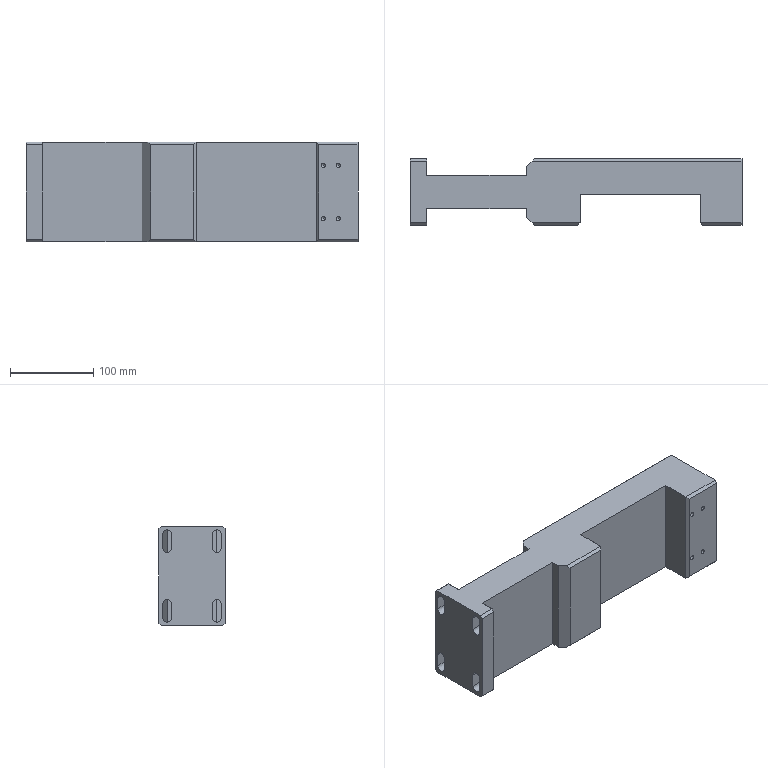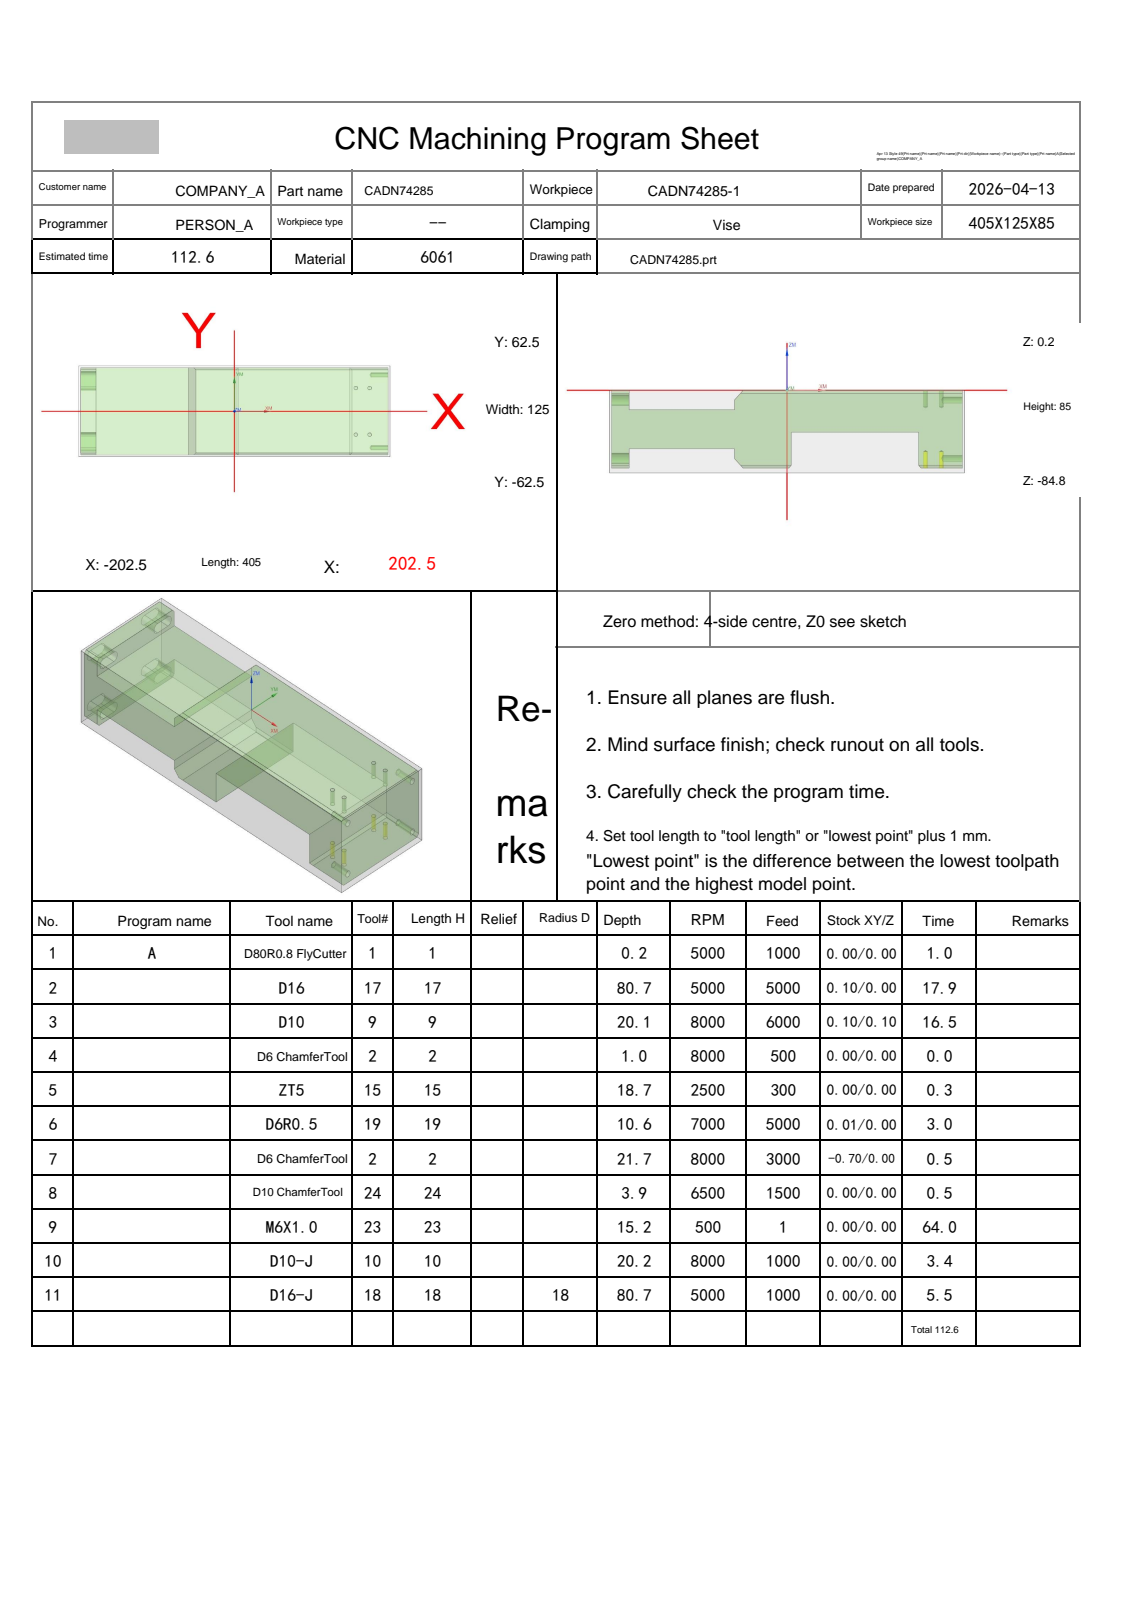NC program | NX | posted by the shop | part box 400 x 80 x 120 mm
Lines 1 to 710 of 8047:
%
O0001
(Machine time: 174.87 MIN)
(===Total Tool:10===)
(T1=D80R0.8 FlyCutter D=80.  R=0.8  D-  H01 Z=-0.   )
(T17=D16    D=16.  R=0.   D-  H17 Z=-80.5 )
(T9=D10     D=10.  R=0.   D-  H09 Z=-19.9 )
(T2=D6 ChamferTool   D=6.   R=0.   D-  H02 Z=-21.5 )
(T15=ZT5    D=5.   DR_a=118 D-  H15 Z=-18.5 )
(T19=D6R0.5 D=6.   R=0.5  D-  H19 Z=-10.4 )
(T24=D10 ChamferTool D=10.  R=0.   D-  H24 Z=-3.7  )
(T23=M6X1.0 D=5.   DR_a=180 D-  H23 Z=-15.  )
(T10=D10-J  D=10.  R=0.   D10 H10 Z=-20.  )
(T18=D16-J  D=16.  R=0.   D18 H18 Z=-80.5 )
G80 G90 G17 G49 G40
G91 G28 Z0
M01
N1 T01 M06
(D80R0.8 FlyCutter  D=80. R=0.8 H=01 ce=0.00 di=0.00)
G00 G90 G54 X245. Y-33.333 M03 S5000
G43 H01 Z20.
M08
Z2.
G01 Z0.0 F1000.
X240.
X-240.
Y33.333
X240.
X245.
Z2.
G00 Z20.
G91 G28 Z0.0
M05
M09
G91 G28 Z0.0
M01
N2 T17 M06
(D16  D=16. R=0. H=17 ce=0.10 di=0.00)
G00 G90 G54 X0.0 Y68.1 M03 S5000
G43 H17 Z20.
M08
Z.5
G01 X200. Z.317 F5000.
G02 X208.1 Y60. Z.305 I0.0 J-8.1
G01 Y-60. Z.195
G02 X200. Y-68.1 Z.183 I-8.1 J0.0
G01 X-200. Z-.183
G02 X-208.1 Y-60. Z-.195 I0.0 J8.1
G01 Y60. Z-.305
G02 X-200. Y68.1 Z-.317 I8.1 J0.0
G01 X200. Z-.683
G02 X208.1 Y60. Z-.695 I0.0 J-8.1
G01 Y-60. Z-.805
G02 X200. Y-68.1 Z-.817 I-8.1 J0.0
G01 X-200. Z-1.183
G02 X-208.1 Y-60. Z-1.195 I0.0 J8.1
G01 Y60. Z-1.305
G02 X-200. Y68.1 Z-1.317 I8.1 J0.0
G01 X200. Z-1.683
G02 X208.1 Y60. Z-1.695 I0.0 J-8.1
G01 Y-60. Z-1.805
G02 X200. Y-68.1 Z-1.817 I-8.1 J0.0
G01 X-200. Z-2.183
G02 X-208.1 Y-60. Z-2.195 I0.0 J8.1
G01 Y60. Z-2.305
G02 X-200. Y68.1 Z-2.317 I8.1 J0.0
G01 X200. Z-2.683
G02 X208.1 Y60. Z-2.695 I0.0 J-8.1
G01 Y-60. Z-2.805
G02 X200. Y-68.1 Z-2.817 I-8.1 J0.0
G01 X-200. Z-3.183
G02 X-208.1 Y-60. Z-3.195 I0.0 J8.1
G01 Y60. Z-3.305
G02 X-200. Y68.1 Z-3.317 I8.1 J0.0
G01 X200. Z-3.683
G02 X208.1 Y60. Z-3.695 I0.0 J-8.1
G01 Y-60. Z-3.805
G02 X200. Y-68.1 Z-3.817 I-8.1 J0.0
G01 X-200. Z-4.183
G02 X-208.1 Y-60. Z-4.195 I0.0 J8.1
G01 Y60. Z-4.305
G02 X-200. Y68.1 Z-4.317 I8.1 J0.0
G01 X200. Z-4.683
G02 X208.1 Y60. Z-4.695 I0.0 J-8.1
G01 Y-60. Z-4.805
G02 X200. Y-68.1 Z-4.817 I-8.1 J0.0
G01 X-200. Z-5.183
G02 X-208.1 Y-60. Z-5.195 I0.0 J8.1
G01 Y60. Z-5.305
G02 X-200. Y68.1 Z-5.317 I8.1 J0.0
G01 X200. Z-5.683
G02 X208.1 Y60. Z-5.695 I0.0 J-8.1
G01 Y-60. Z-5.805
G02 X200. Y-68.1 Z-5.817 I-8.1 J0.0
G01 X-200. Z-6.183
G02 X-208.1 Y-60. Z-6.195 I0.0 J8.1
G01 Y60. Z-6.305
G02 X-200. Y68.1 Z-6.317 I8.1 J0.0
G01 X200. Z-6.683
G02 X208.1 Y60. Z-6.695 I0.0 J-8.1
G01 Y-60. Z-6.805
G02 X200. Y-68.1 Z-6.817 I-8.1 J0.0
G01 X-200. Z-7.183
G02 X-208.1 Y-60. Z-7.195 I0.0 J8.1
G01 Y60. Z-7.305
G02 X-200. Y68.1 Z-7.317 I8.1 J0.0
G01 X200. Z-7.683
G02 X208.1 Y60. Z-7.695 I0.0 J-8.1
G01 Y-60. Z-7.805
G02 X200. Y-68.1 Z-7.817 I-8.1 J0.0
G01 X-200. Z-8.183
G02 X-208.1 Y-60. Z-8.195 I0.0 J8.1
G01 Y60. Z-8.305
G02 X-200. Y68.1 Z-8.317 I8.1 J0.0
G01 X200. Z-8.683
G02 X208.1 Y60. Z-8.695 I0.0 J-8.1
G01 Y-60. Z-8.805
G02 X200. Y-68.1 Z-8.817 I-8.1 J0.0
G01 X-200. Z-9.183
G02 X-208.1 Y-60. Z-9.195 I0.0 J8.1
G01 Y60. Z-9.305
G02 X-200. Y68.1 Z-9.317 I8.1 J0.0
G01 X200. Z-9.683
G02 X208.1 Y60. Z-9.695 I0.0 J-8.1
G01 Y-60. Z-9.805
G02 X200. Y-68.1 Z-9.817 I-8.1 J0.0
G01 X-200. Z-10.183
G02 X-208.1 Y-60. Z-10.195 I0.0 J8.1
G01 Y60. Z-10.305
G02 X-200. Y68.1 Z-10.317 I8.1 J0.0
G01 X200. Z-10.683
G02 X208.1 Y60. Z-10.695 I0.0 J-8.1
G01 Y-60. Z-10.805
G02 X200. Y-68.1 Z-10.817 I-8.1 J0.0
G01 X-200. Z-11.183
G02 X-208.1 Y-60. Z-11.195 I0.0 J8.1
G01 Y60. Z-11.305
G02 X-200. Y68.1 Z-11.317 I8.1 J0.0
G01 X200. Z-11.683
G02 X208.1 Y60. Z-11.695 I0.0 J-8.1
G01 Y-60. Z-11.805
G02 X200. Y-68.1 Z-11.817 I-8.1 J0.0
G01 X-200. Z-12.183
G02 X-208.1 Y-60. Z-12.195 I0.0 J8.1
G01 Y60. Z-12.305
G02 X-200. Y68.1 Z-12.317 I8.1 J0.0
G01 X200. Z-12.683
G02 X208.1 Y60. Z-12.695 I0.0 J-8.1
G01 Y-60. Z-12.805
G02 X200. Y-68.1 Z-12.817 I-8.1 J0.0
G01 X-200. Z-13.183
G02 X-208.1 Y-60. Z-13.195 I0.0 J8.1
G01 Y60. Z-13.305
G02 X-200. Y68.1 Z-13.317 I8.1 J0.0
G01 X200. Z-13.683
G02 X208.1 Y60. Z-13.695 I0.0 J-8.1
G01 Y-60. Z-13.805
G02 X200. Y-68.1 Z-13.817 I-8.1 J0.0
G01 X-200. Z-14.183
G02 X-208.1 Y-60. Z-14.195 I0.0 J8.1
G01 Y60. Z-14.305
G02 X-200. Y68.1 Z-14.317 I8.1 J0.0
G01 X200. Z-14.683
G02 X208.1 Y60. Z-14.695 I0.0 J-8.1
G01 Y-60. Z-14.805
G02 X200. Y-68.1 Z-14.817 I-8.1 J0.0
G01 X-200. Z-15.183
G02 X-208.1 Y-60. Z-15.195 I0.0 J8.1
G01 Y60. Z-15.305
G02 X-200. Y68.1 Z-15.317 I8.1 J0.0
G01 X200. Z-15.683
G02 X208.1 Y60. Z-15.695 I0.0 J-8.1
G01 Y-60. Z-15.805
G02 X200. Y-68.1 Z-15.817 I-8.1 J0.0
G01 X-200. Z-16.183
G02 X-208.1 Y-60. Z-16.195 I0.0 J8.1
G01 Y60. Z-16.305
G02 X-200. Y68.1 Z-16.317 I8.1 J0.0
G01 X200. Z-16.683
G02 X208.1 Y60. Z-16.695 I0.0 J-8.1
G01 Y-60. Z-16.805
G02 X200. Y-68.1 Z-16.817 I-8.1 J0.0
G01 X-200. Z-17.183
G02 X-208.1 Y-60. Z-17.195 I0.0 J8.1
G01 Y60. Z-17.305
G02 X-200. Y68.1 Z-17.317 I8.1 J0.0
G01 X200. Z-17.683
G02 X208.1 Y60. Z-17.695 I0.0 J-8.1
G01 Y-60. Z-17.805
G02 X200. Y-68.1 Z-17.817 I-8.1 J0.0
G01 X-200. Z-18.183
G02 X-208.1 Y-60. Z-18.195 I0.0 J8.1
G01 Y60. Z-18.305
G02 X-200. Y68.1 Z-18.317 I8.1 J0.0
G01 X200. Z-18.683
G02 X208.1 Y60. Z-18.695 I0.0 J-8.1
G01 Y-60. Z-18.805
G02 X200. Y-68.1 Z-18.817 I-8.1 J0.0
G01 X-200. Z-19.183
G02 X-208.1 Y-60. Z-19.195 I0.0 J8.1
G01 Y60. Z-19.305
G02 X-200. Y68.1 Z-19.317 I8.1 J0.0
G01 X200. Z-19.683
G02 X208.1 Y60. Z-19.695 I0.0 J-8.1
G01 Y-60. Z-19.805
G02 X200. Y-68.1 Z-19.817 I-8.1 J0.0
G01 X-200. Z-20.183
G02 X-208.1 Y-60. Z-20.195 I0.0 J8.1
G01 Y60. Z-20.305
G02 X-200. Y68.1 Z-20.317 I8.1 J0.0
G01 X200. Z-20.683
G02 X208.1 Y60. Z-20.695 I0.0 J-8.1
G01 Y-60. Z-20.805
G02 X200. Y-68.1 Z-20.817 I-8.1 J0.0
G01 X-200. Z-21.183
G02 X-208.1 Y-60. Z-21.195 I0.0 J8.1
G01 Y60. Z-21.305
G02 X-200. Y68.1 Z-21.317 I8.1 J0.0
G01 X200. Z-21.683
G02 X208.1 Y60. Z-21.695 I0.0 J-8.1
G01 Y-60. Z-21.805
G02 X200. Y-68.1 Z-21.817 I-8.1 J0.0
G01 X-200. Z-22.183
G02 X-208.1 Y-60. Z-22.195 I0.0 J8.1
G01 Y60. Z-22.305
G02 X-200. Y68.1 Z-22.317 I8.1 J0.0
G01 X200. Z-22.683
G02 X208.1 Y60. Z-22.695 I0.0 J-8.1
G01 Y-60. Z-22.805
G02 X200. Y-68.1 Z-22.817 I-8.1 J0.0
G01 X-200. Z-23.183
G02 X-208.1 Y-60. Z-23.195 I0.0 J8.1
G01 Y60. Z-23.305
G02 X-200. Y68.1 Z-23.317 I8.1 J0.0
G01 X200. Z-23.683
G02 X208.1 Y60. Z-23.695 I0.0 J-8.1
G01 Y-60. Z-23.805
G02 X200. Y-68.1 Z-23.817 I-8.1 J0.0
G01 X-200. Z-24.183
G02 X-208.1 Y-60. Z-24.195 I0.0 J8.1
G01 Y60. Z-24.305
G02 X-200. Y68.1 Z-24.317 I8.1 J0.0
G01 X200. Z-24.683
G02 X208.1 Y60. Z-24.695 I0.0 J-8.1
G01 Y-60. Z-24.805
G02 X200. Y-68.1 Z-24.817 I-8.1 J0.0
G01 X-200. Z-25.183
G02 X-208.1 Y-60. Z-25.195 I0.0 J8.1
G01 Y60. Z-25.305
G02 X-200. Y68.1 Z-25.317 I8.1 J0.0
G01 X200. Z-25.683
G02 X208.1 Y60. Z-25.695 I0.0 J-8.1
G01 Y-60. Z-25.805
G02 X200. Y-68.1 Z-25.817 I-8.1 J0.0
G01 X-200. Z-26.183
G02 X-208.1 Y-60. Z-26.195 I0.0 J8.1
G01 Y60. Z-26.305
G02 X-200. Y68.1 Z-26.317 I8.1 J0.0
G01 X200. Z-26.683
G02 X208.1 Y60. Z-26.695 I0.0 J-8.1
G01 Y-60. Z-26.805
G02 X200. Y-68.1 Z-26.817 I-8.1 J0.0
G01 X-200. Z-27.183
G02 X-208.1 Y-60. Z-27.195 I0.0 J8.1
G01 Y60. Z-27.305
G02 X-200. Y68.1 Z-27.317 I8.1 J0.0
G01 X200. Z-27.683
G02 X208.1 Y60. Z-27.695 I0.0 J-8.1
G01 Y-60. Z-27.805
G02 X200. Y-68.1 Z-27.817 I-8.1 J0.0
G01 X-200. Z-28.183
G02 X-208.1 Y-60. Z-28.195 I0.0 J8.1
G01 Y60. Z-28.305
G02 X-200. Y68.1 Z-28.317 I8.1 J0.0
G01 X200. Z-28.683
G02 X208.1 Y60. Z-28.695 I0.0 J-8.1
G01 Y-60. Z-28.805
G02 X200. Y-68.1 Z-28.817 I-8.1 J0.0
G01 X-200. Z-29.183
G02 X-208.1 Y-60. Z-29.195 I0.0 J8.1
G01 Y60. Z-29.305
G02 X-200. Y68.1 Z-29.317 I8.1 J0.0
G01 X200. Z-29.683
G02 X208.1 Y60. Z-29.695 I0.0 J-8.1
G01 Y-60. Z-29.805
G02 X200. Y-68.1 Z-29.817 I-8.1 J0.0
G01 X-200. Z-30.183
G02 X-208.1 Y-60. Z-30.195 I0.0 J8.1
G01 Y60. Z-30.305
G02 X-200. Y68.1 Z-30.317 I8.1 J0.0
G01 X200. Z-30.683
G02 X208.1 Y60. Z-30.695 I0.0 J-8.1
G01 Y-60. Z-30.805
G02 X200. Y-68.1 Z-30.817 I-8.1 J0.0
G01 X-200. Z-31.183
G02 X-208.1 Y-60. Z-31.195 I0.0 J8.1
G01 Y60. Z-31.305
G02 X-200. Y68.1 Z-31.317 I8.1 J0.0
G01 X200. Z-31.683
G02 X208.1 Y60. Z-31.695 I0.0 J-8.1
G01 Y-60. Z-31.805
G02 X200. Y-68.1 Z-31.817 I-8.1 J0.0
G01 X-200. Z-32.183
G02 X-208.1 Y-60. Z-32.195 I0.0 J8.1
G01 Y60. Z-32.305
G02 X-200. Y68.1 Z-32.317 I8.1 J0.0
G01 X200. Z-32.683
G02 X208.1 Y60. Z-32.695 I0.0 J-8.1
G01 Y-60. Z-32.805
G02 X200. Y-68.1 Z-32.817 I-8.1 J0.0
G01 X-200. Z-33.183
G02 X-208.1 Y-60. Z-33.195 I0.0 J8.1
G01 Y60. Z-33.305
G02 X-200. Y68.1 Z-33.317 I8.1 J0.0
G01 X200. Z-33.683
G02 X208.1 Y60. Z-33.695 I0.0 J-8.1
G01 Y-60. Z-33.805
G02 X200. Y-68.1 Z-33.817 I-8.1 J0.0
G01 X-200. Z-34.183
G02 X-208.1 Y-60. Z-34.195 I0.0 J8.1
G01 Y60. Z-34.305
G02 X-200. Y68.1 Z-34.317 I8.1 J0.0
G01 X200. Z-34.683
G02 X208.1 Y60. Z-34.695 I0.0 J-8.1
G01 Y-60. Z-34.805
G02 X200. Y-68.1 Z-34.817 I-8.1 J0.0
G01 X-200. Z-35.183
G02 X-208.1 Y-60. Z-35.195 I0.0 J8.1
G01 Y60. Z-35.305
G02 X-200. Y68.1 Z-35.317 I8.1 J0.0
G01 X200. Z-35.683
G02 X208.1 Y60. Z-35.695 I0.0 J-8.1
G01 Y-60. Z-35.805
G02 X200. Y-68.1 Z-35.817 I-8.1 J0.0
G01 X-200. Z-36.183
G02 X-208.1 Y-60. Z-36.195 I0.0 J8.1
G01 Y60. Z-36.305
G02 X-200. Y68.1 Z-36.317 I8.1 J0.0
G01 X200. Z-36.683
G02 X208.1 Y60. Z-36.695 I0.0 J-8.1
G01 Y-60. Z-36.805
G02 X200. Y-68.1 Z-36.817 I-8.1 J0.0
G01 X-200. Z-37.183
G02 X-208.1 Y-60. Z-37.195 I0.0 J8.1
G01 Y60. Z-37.305
G02 X-200. Y68.1 Z-37.317 I8.1 J0.0
G01 X200. Z-37.683
G02 X208.1 Y60. Z-37.695 I0.0 J-8.1
G01 Y-60. Z-37.805
G02 X200. Y-68.1 Z-37.817 I-8.1 J0.0
G01 X-200. Z-38.183
G02 X-208.1 Y-60. Z-38.195 I0.0 J8.1
G01 Y60. Z-38.305
G02 X-200. Y68.1 Z-38.317 I8.1 J0.0
G01 X200. Z-38.683
G02 X208.1 Y60. Z-38.695 I0.0 J-8.1
G01 Y-60. Z-38.805
G02 X200. Y-68.1 Z-38.817 I-8.1 J0.0
G01 X-200. Z-39.183
G02 X-208.1 Y-60. Z-39.195 I0.0 J8.1
G01 Y60. Z-39.305
G02 X-200. Y68.1 Z-39.317 I8.1 J0.0
G01 X200. Z-39.683
G02 X208.1 Y60. Z-39.695 I0.0 J-8.1
G01 Y-60. Z-39.805
G02 X200. Y-68.1 Z-39.817 I-8.1 J0.0
G01 X-200. Z-40.183
G02 X-208.1 Y-60. Z-40.195 I0.0 J8.1
G01 Y60. Z-40.305
G02 X-200. Y68.1 Z-40.317 I8.1 J0.0
G01 X200. Z-40.683
G02 X208.1 Y60. Z-40.695 I0.0 J-8.1
G01 Y-60. Z-40.805
G02 X200. Y-68.1 Z-40.817 I-8.1 J0.0
G01 X-200. Z-41.183
G02 X-208.1 Y-60. Z-41.195 I0.0 J8.1
G01 Y60. Z-41.305
G02 X-200. Y68.1 Z-41.317 I8.1 J0.0
G01 X200. Z-41.683
G02 X208.1 Y60. Z-41.695 I0.0 J-8.1
G01 Y-60. Z-41.805
G02 X200. Y-68.1 Z-41.817 I-8.1 J0.0
G01 X-200. Z-42.183
G02 X-208.1 Y-60. Z-42.195 I0.0 J8.1
G01 Y60. Z-42.305
G02 X-200. Y68.1 Z-42.317 I8.1 J0.0
G01 X200. Z-42.683
G02 X208.1 Y60. Z-42.695 I0.0 J-8.1
G01 Y-60. Z-42.805
G02 X200. Y-68.1 Z-42.817 I-8.1 J0.0
G01 X-200. Z-43.183
G02 X-208.1 Y-60. Z-43.195 I0.0 J8.1
G01 Y60. Z-43.305
G02 X-200. Y68.1 Z-43.317 I8.1 J0.0
G01 X200. Z-43.683
G02 X208.1 Y60. Z-43.695 I0.0 J-8.1
G01 Y-60. Z-43.805
G02 X200. Y-68.1 Z-43.817 I-8.1 J0.0
G01 X-200. Z-44.183
G02 X-208.1 Y-60. Z-44.195 I0.0 J8.1
G01 Y60. Z-44.305
G02 X-200. Y68.1 Z-44.317 I8.1 J0.0
G01 X200. Z-44.683
G02 X208.1 Y60. Z-44.695 I0.0 J-8.1
G01 Y-60. Z-44.805
G02 X200. Y-68.1 Z-44.817 I-8.1 J0.0
G01 X-200. Z-45.183
G02 X-208.1 Y-60. Z-45.195 I0.0 J8.1
G01 Y60. Z-45.305
G02 X-200. Y68.1 Z-45.317 I8.1 J0.0
G01 X200. Z-45.683
G02 X208.1 Y60. Z-45.695 I0.0 J-8.1
G01 Y-60. Z-45.805
G02 X200. Y-68.1 Z-45.817 I-8.1 J0.0
G01 X-200. Z-46.183
G02 X-208.1 Y-60. Z-46.195 I0.0 J8.1
G01 Y60. Z-46.305
G02 X-200. Y68.1 Z-46.317 I8.1 J0.0
G01 X200. Z-46.683
G02 X208.1 Y60. Z-46.695 I0.0 J-8.1
G01 Y-60. Z-46.805
G02 X200. Y-68.1 Z-46.817 I-8.1 J0.0
G01 X-200. Z-47.183
G02 X-208.1 Y-60. Z-47.195 I0.0 J8.1
G01 Y60. Z-47.305
G02 X-200. Y68.1 Z-47.317 I8.1 J0.0
G01 X200. Z-47.683
G02 X208.1 Y60. Z-47.695 I0.0 J-8.1
G01 Y-60. Z-47.805
G02 X200. Y-68.1 Z-47.817 I-8.1 J0.0
G01 X-200. Z-48.183
G02 X-208.1 Y-60. Z-48.195 I0.0 J8.1
G01 Y60. Z-48.305
G02 X-200. Y68.1 Z-48.317 I8.1 J0.0
G01 X200. Z-48.683
G02 X208.1 Y60. Z-48.695 I0.0 J-8.1
G01 Y-60. Z-48.805
G02 X200. Y-68.1 Z-48.817 I-8.1 J0.0
G01 X-200. Z-49.183
G02 X-208.1 Y-60. Z-49.195 I0.0 J8.1
G01 Y60. Z-49.305
G02 X-200. Y68.1 Z-49.317 I8.1 J0.0
G01 X200. Z-49.683
G02 X208.1 Y60. Z-49.695 I0.0 J-8.1
G01 Y-60. Z-49.805
G02 X200. Y-68.1 Z-49.817 I-8.1 J0.0
G01 X-200. Z-50.183
G02 X-208.1 Y-60. Z-50.195 I0.0 J8.1
G01 Y60. Z-50.305
G02 X-200. Y68.1 Z-50.317 I8.1 J0.0
G01 X200. Z-50.683
G02 X208.1 Y60. Z-50.695 I0.0 J-8.1
G01 Y-60. Z-50.805
G02 X200. Y-68.1 Z-50.817 I-8.1 J0.0
G01 X-200. Z-51.183
G02 X-208.1 Y-60. Z-51.195 I0.0 J8.1
G01 Y60. Z-51.305
G02 X-200. Y68.1 Z-51.317 I8.1 J0.0
G01 X200. Z-51.683
G02 X208.1 Y60. Z-51.695 I0.0 J-8.1
G01 Y-60. Z-51.805
G02 X200. Y-68.1 Z-51.817 I-8.1 J0.0
G01 X-200. Z-52.183
G02 X-208.1 Y-60. Z-52.195 I0.0 J8.1
G01 Y60. Z-52.305
G02 X-200. Y68.1 Z-52.317 I8.1 J0.0
G01 X200. Z-52.683
G02 X208.1 Y60. Z-52.695 I0.0 J-8.1
G01 Y-60. Z-52.805
G02 X200. Y-68.1 Z-52.817 I-8.1 J0.0
G01 X-200. Z-53.183
G02 X-208.1 Y-60. Z-53.195 I0.0 J8.1
G01 Y60. Z-53.305
G02 X-200. Y68.1 Z-53.317 I8.1 J0.0
G01 X200. Z-53.683
G02 X208.1 Y60. Z-53.695 I0.0 J-8.1
G01 Y-60. Z-53.805
G02 X200. Y-68.1 Z-53.817 I-8.1 J0.0
G01 X-200. Z-54.183
G02 X-208.1 Y-60. Z-54.195 I0.0 J8.1
G01 Y60. Z-54.305
G02 X-200. Y68.1 Z-54.317 I8.1 J0.0
G01 X200. Z-54.683
G02 X208.1 Y60. Z-54.695 I0.0 J-8.1
G01 Y-60. Z-54.805
G02 X200. Y-68.1 Z-54.817 I-8.1 J0.0
G01 X-200. Z-55.183
G02 X-208.1 Y-60. Z-55.195 I0.0 J8.1
G01 Y60. Z-55.305
G02 X-200. Y68.1 Z-55.317 I8.1 J0.0
G01 X200. Z-55.683
G02 X208.1 Y60. Z-55.695 I0.0 J-8.1
G01 Y-60. Z-55.805
G02 X200. Y-68.1 Z-55.817 I-8.1 J0.0
G01 X-200. Z-56.183
G02 X-208.1 Y-60. Z-56.195 I0.0 J8.1
G01 Y60. Z-56.305
G02 X-200. Y68.1 Z-56.317 I8.1 J0.0
G01 X200. Z-56.683
G02 X208.1 Y60. Z-56.695 I0.0 J-8.1
G01 Y-60. Z-56.805
G02 X200. Y-68.1 Z-56.817 I-8.1 J0.0
G01 X-200. Z-57.183
G02 X-208.1 Y-60. Z-57.195 I0.0 J8.1
G01 Y60. Z-57.305
G02 X-200. Y68.1 Z-57.317 I8.1 J0.0
G01 X200. Z-57.683
G02 X208.1 Y60. Z-57.695 I0.0 J-8.1
G01 Y-60. Z-57.805
G02 X200. Y-68.1 Z-57.817 I-8.1 J0.0
G01 X-200. Z-58.183
G02 X-208.1 Y-60. Z-58.195 I0.0 J8.1
G01 Y60. Z-58.305
G02 X-200. Y68.1 Z-58.317 I8.1 J0.0
G01 X200. Z-58.683
G02 X208.1 Y60. Z-58.695 I0.0 J-8.1
G01 Y-60. Z-58.805
G02 X200. Y-68.1 Z-58.817 I-8.1 J0.0
G01 X-200. Z-59.183
G02 X-208.1 Y-60. Z-59.195 I0.0 J8.1
G01 Y60. Z-59.305
G02 X-200. Y68.1 Z-59.317 I8.1 J0.0
G01 X200. Z-59.683
G02 X208.1 Y60. Z-59.695 I0.0 J-8.1
G01 Y-60. Z-59.805
G02 X200. Y-68.1 Z-59.817 I-8.1 J0.0
G01 X-200. Z-60.183
G02 X-208.1 Y-60. Z-60.195 I0.0 J8.1
G01 Y60. Z-60.305
G02 X-200. Y68.1 Z-60.317 I8.1 J0.0
G01 X200. Z-60.683
G02 X208.1 Y60. Z-60.695 I0.0 J-8.1
G01 Y-60. Z-60.805
G02 X200. Y-68.1 Z-60.817 I-8.1 J0.0
G01 X-200. Z-61.183
G02 X-208.1 Y-60. Z-61.195 I0.0 J8.1
G01 Y60. Z-61.305
G02 X-200. Y68.1 Z-61.317 I8.1 J0.0
G01 X200. Z-61.683
G02 X208.1 Y60. Z-61.695 I0.0 J-8.1
G01 Y-60. Z-61.805
G02 X200. Y-68.1 Z-61.817 I-8.1 J0.0
G01 X-200. Z-62.183
G02 X-208.1 Y-60. Z-62.195 I0.0 J8.1
G01 Y60. Z-62.305
G02 X-200. Y68.1 Z-62.317 I8.1 J0.0
G01 X200. Z-62.683
G02 X208.1 Y60. Z-62.695 I0.0 J-8.1
G01 Y-60. Z-62.805
G02 X200. Y-68.1 Z-62.817 I-8.1 J0.0
G01 X-200. Z-63.183
G02 X-208.1 Y-60. Z-63.195 I0.0 J8.1
G01 Y60. Z-63.305
G02 X-200. Y68.1 Z-63.317 I8.1 J0.0
G01 X200. Z-63.683
G02 X208.1 Y60. Z-63.695 I0.0 J-8.1
G01 Y-60. Z-63.805
G02 X200. Y-68.1 Z-63.817 I-8.1 J0.0
G01 X-200. Z-64.183
G02 X-208.1 Y-60. Z-64.195 I0.0 J8.1
G01 Y60. Z-64.305
G02 X-200. Y68.1 Z-64.317 I8.1 J0.0
G01 X200. Z-64.683
G02 X208.1 Y60. Z-64.695 I0.0 J-8.1
G01 Y-60. Z-64.805
G02 X200. Y-68.1 Z-64.817 I-8.1 J0.0
G01 X-200. Z-65.183
G02 X-208.1 Y-60. Z-65.195 I0.0 J8.1
G01 Y60. Z-65.305
G02 X-200. Y68.1 Z-65.317 I8.1 J0.0
G01 X200. Z-65.683
G02 X208.1 Y60. Z-65.695 I0.0 J-8.1
G01 Y-60. Z-65.805
G02 X200. Y-68.1 Z-65.817 I-8.1 J0.0
G01 X-200. Z-66.183
G02 X-208.1 Y-60. Z-66.195 I0.0 J8.1
G01 Y60. Z-66.305
G02 X-200. Y68.1 Z-66.317 I8.1 J0.0
G01 X200. Z-66.683
G02 X208.1 Y60. Z-66.695 I0.0 J-8.1
G01 Y-60. Z-66.805
G02 X200. Y-68.1 Z-66.817 I-8.1 J0.0
G01 X-200. Z-67.183
G02 X-208.1 Y-60. Z-67.195 I0.0 J8.1
G01 Y60. Z-67.305
G02 X-200. Y68.1 Z-67.317 I8.1 J0.0
G01 X200. Z-67.683
G02 X208.1 Y60. Z-67.695 I0.0 J-8.1
G01 Y-60. Z-67.805
G02 X200. Y-68.1 Z-67.817 I-8.1 J0.0
G01 X-200. Z-68.183
G02 X-208.1 Y-60. Z-68.195 I0.0 J8.1
G01 Y60. Z-68.305
G02 X-200. Y68.1 Z-68.317 I8.1 J0.0
G01 X200. Z-68.683
G02 X208.1 Y60. Z-68.695 I0.0 J-8.1
G01 Y-60. Z-68.805
G02 X200. Y-68.1 Z-68.817 I-8.1 J0.0
G01 X-200. Z-69.183
G02 X-208.1 Y-60. Z-69.195 I0.0 J8.1
G01 Y60. Z-69.305
G02 X-200. Y68.1 Z-69.317 I8.1 J0.0
G01 X200. Z-69.683
G02 X208.1 Y60. Z-69.695 I0.0 J-8.1
G01 Y-60. Z-69.805
G02 X200. Y-68.1 Z-69.817 I-8.1 J0.0
G01 X-200. Z-70.183
G02 X-208.1 Y-60. Z-70.195 I0.0 J8.1
G01 Y60. Z-70.305
G02 X-200. Y68.1 Z-70.317 I8.1 J0.0
G01 X200. Z-70.683
G02 X208.1 Y60. Z-70.695 I0.0 J-8.1
G01 Y-60. Z-70.805
G02 X200. Y-68.1 Z-70.817 I-8.1 J0.0
G01 X-200. Z-71.183
G02 X-208.1 Y-60. Z-71.195 I0.0 J8.1
G01 Y60. Z-71.305
G02 X-200. Y68.1 Z-71.317 I8.1 J0.0
G01 X200. Z-71.683
G02 X208.1 Y60. Z-71.695 I0.0 J-8.1
G01 Y-60. Z-71.805
G02 X200. Y-68.1 Z-71.817 I-8.1 J0.0
G01 X-200. Z-72.183
G02 X-208.1 Y-60. Z-72.195 I0.0 J8.1
G01 Y60. Z-72.305
G02 X-200. Y68.1 Z-72.317 I8.1 J0.0
G01 X200. Z-72.683
G02 X208.1 Y60. Z-72.695 I0.0 J-8.1
G01 Y-60. Z-72.805
G02 X200. Y-68.1 Z-72.817 I-8.1 J0.0
G01 X-200. Z-73.183
G02 X-208.1 Y-60. Z-73.195 I0.0 J8.1
G01 Y60. Z-73.305
G02 X-200. Y68.1 Z-73.317 I8.1 J0.0
G01 X200. Z-73.683
G02 X208.1 Y60. Z-73.695 I0.0 J-8.1
G01 Y-60. Z-73.805
G02 X200. Y-68.1 Z-73.817 I-8.1 J0.0
G01 X-200. Z-74.183
G02 X-208.1 Y-60. Z-74.195 I0.0 J8.1
G01 Y60. Z-74.305
G02 X-200. Y68.1 Z-74.317 I8.1 J0.0
G01 X200. Z-74.683
G02 X208.1 Y60. Z-74.695 I0.0 J-8.1
G01 Y-60. Z-74.805
G02 X200. Y-68.1 Z-74.817 I-8.1 J0.0
G01 X-200. Z-75.183
G02 X-208.1 Y-60. Z-75.195 I0.0 J8.1
G01 Y60. Z-75.305
G02 X-200. Y68.1 Z-75.317 I8.1 J0.0
G01 X200. Z-75.683
G02 X208.1 Y60. Z-75.695 I0.0 J-8.1
G01 Y-60. Z-75.805
G02 X200. Y-68.1 Z-75.817 I-8.1 J0.0
G01 X-200. Z-76.183
G02 X-208.1 Y-60. Z-76.195 I0.0 J8.1
G01 Y60. Z-76.305
G02 X-200. Y68.1 Z-76.317 I8.1 J0.0
G01 X200. Z-76.683
G02 X208.1 Y60. Z-76.695 I0.0 J-8.1
G01 Y-60. Z-76.805
G02 X200. Y-68.1 Z-76.817 I-8.1 J0.0
G01 X-200. Z-77.183
G02 X-208.1 Y-60. Z-77.195 I0.0 J8.1
G01 Y60. Z-77.305
G02 X-200. Y68.1 Z-77.317 I8.1 J0.0
G01 X200. Z-77.683
G02 X208.1 Y60. Z-77.695 I0.0 J-8.1
G01 Y-60. Z-77.805
G02 X200. Y-68.1 Z-77.817 I-8.1 J0.0
G01 X-200. Z-78.183
G02 X-208.1 Y-60. Z-78.195 I0.0 J8.1
G01 Y60. Z-78.305
G02 X-200. Y68.1 Z-78.317 I8.1 J0.0
G01 X200. Z-78.683
G02 X208.1 Y60. Z-78.695 I0.0 J-8.1
G01 Y-60. Z-78.805
G02 X200. Y-68.1 Z-78.817 I-8.1 J0.0
G01 X-200. Z-79.183
G02 X-208.1 Y-60. Z-79.195 I0.0 J8.1
G01 Y60. Z-79.305
G02 X-200. Y68.1 Z-79.317 I8.1 J0.0
G01 X200. Z-79.683
G02 X208.1 Y60. Z-79.695 I0.0 J-8.1
G01 Y-60. Z-79.805
G02 X200. Y-68.1 Z-79.817 I-8.1 J0.0
G01 X-200. Z-80.183
G02 X-208.1 Y-60. Z-80.195 I0.0 J8.1
G01 Y60. Z-80.305
G02 X-200. Y68.1 Z-80.317 I8.1 J0.0
G01 X0.0 Z-80.5
X200.
G02 X208.1 Y60. I0.0 J-8.1
G01 Y-60.
G02 X200. Y-68.1 I-8.1 J0.0
G01 X-200.
G02 X-208.1 Y-60. I0.0 J8.1
G01 Y60.
G02 X-200. Y68.1 I8.1 J0.0
G01 X0.0
X.5
Z-79.5
G00 Z20.
G91 G28 Z0.0
M05
M09
G91 G28 Z0.0
M01